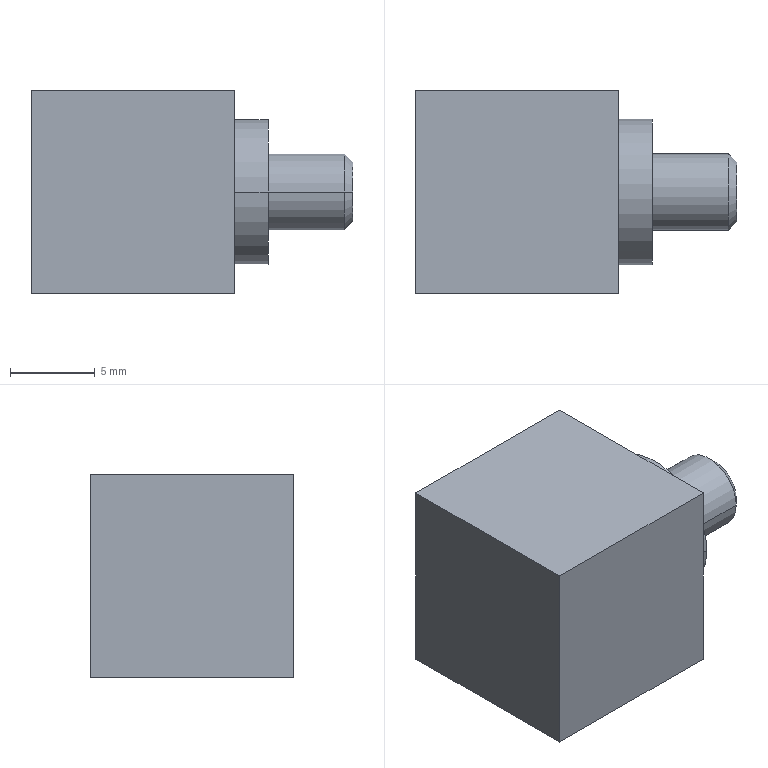Part | STEP file | [LF-A(SUS)]-4 | 1 solid | 23 faces | box 19 x 12 x 12 mm | volume 1287 mm3 | plane 9 | cone 8 | cylinder 6 | commonest cylinder face diameters 4.5 x2 8.6 x2 9.2 x2
STEP:
#1=CARTESIAN_POINT('',(0.,0.,0.));
#2=DIRECTION('',(0.,0.,1.));
#3=DIRECTION('',(1.,0.,0.));
#4=AXIS2_PLACEMENT_3D('',#1,#2,#3);
#5=CARTESIAN_POINT('',(19.,4.25,6.));
#6=VERTEX_POINT('',#5);
#7=CARTESIAN_POINT('',(19.,7.75,6.));
#8=VERTEX_POINT('',#7);
#9=CARTESIAN_POINT('',(19.,6.,6.));
#10=DIRECTION('',(1.,0.,0.));
#11=DIRECTION('',(0.,-1.,0.));
#12=AXIS2_PLACEMENT_3D('',#9,#10,#11);
#13=CIRCLE('',#12,1.75);
#14=CARTESIAN_POINT('',(18.5,6.,6.));
#15=DIRECTION('',(-1.,0.,0.));
#16=DIRECTION('',(0.,1.,0.));
#17=AXIS2_PLACEMENT_3D('',#14,#15,#16);
#18=CONICAL_SURFACE('',#17,2.25,0.7854);
#19=CARTESIAN_POINT('',(3.142,-0.5));
#20=DIRECTION('',(-1.,0.));
#21=VECTOR('',#20,1.);
#22=LINE('',#19,#21);
#23=(GEOMETRIC_REPRESENTATION_CONTEXT(2)PARAMETRIC_REPRESENTATION_CONTEXT()REPRESENTATION_CONTEXT('',''));
#24=DEFINITIONAL_REPRESENTATION('',(#22),#23);
#25=PCURVE('',#18,#24);
#26=CARTESIAN_POINT('',(19.,6.,6.));
#27=DIRECTION('',(1.,0.,0.));
#28=DIRECTION('',(0.,-1.,0.));
#29=AXIS2_PLACEMENT_3D('',#26,#27,#28);
#30=PLANE('',#29);
#31=CARTESIAN_POINT('',(0.,0.));
#32=DIRECTION('',(1.,0.));
#33=AXIS2_PLACEMENT_2D('',#31,#32);
#34=CIRCLE('',#33,1.75);
#35=(GEOMETRIC_REPRESENTATION_CONTEXT(2)PARAMETRIC_REPRESENTATION_CONTEXT()REPRESENTATION_CONTEXT('',''));
#36=DEFINITIONAL_REPRESENTATION('',(#34),#35);
#37=PCURVE('',#30,#36);
#38=SURFACE_CURVE('',#13,(#25,#37),.PCURVE_S1.);
#39=EDGE_CURVE('',#6,#8,#38,.T.);
#40=ORIENTED_EDGE('',*,*,#39,.F.);
#41=CARTESIAN_POINT('',(18.5,3.75,6.));
#42=VERTEX_POINT('',#41);
#43=CARTESIAN_POINT('',(18.5,3.75,6.));
#44=DIRECTION('',(-0.7071,-0.7071,0.));
#45=VECTOR('',#44,1.);
#46=LINE('',#43,#45);
#47=CARTESIAN_POINT('',(3.142,0.));
#48=DIRECTION('',(0.,1.));
#49=VECTOR('',#48,1.);
#50=LINE('',#47,#49);
#51=(GEOMETRIC_REPRESENTATION_CONTEXT(2)PARAMETRIC_REPRESENTATION_CONTEXT()REPRESENTATION_CONTEXT('',''));
#52=DEFINITIONAL_REPRESENTATION('',(#50),#51);
#53=PCURVE('',#18,#52);
#54=CARTESIAN_POINT('',(18.5,6.,6.));
#55=DIRECTION('',(-1.,0.,0.));
#56=DIRECTION('',(0.,1.,0.));
#57=AXIS2_PLACEMENT_3D('',#54,#55,#56);
#58=CONICAL_SURFACE('',#57,2.25,0.7854);
#59=CARTESIAN_POINT('',(3.142,0.));
#60=DIRECTION('',(0.,1.));
#61=VECTOR('',#60,1.);
#62=LINE('',#59,#61);
#63=(GEOMETRIC_REPRESENTATION_CONTEXT(2)PARAMETRIC_REPRESENTATION_CONTEXT()REPRESENTATION_CONTEXT('',''));
#64=DEFINITIONAL_REPRESENTATION('',(#62),#63);
#65=PCURVE('',#58,#64);
#66=SURFACE_CURVE('',#46,(#53,#65),.PCURVE_S1.);
#67=EDGE_CURVE('',#6,#42,#66,.T.);
#68=ORIENTED_EDGE('',*,*,#67,.T.);
#69=CARTESIAN_POINT('',(18.5,8.25,6.));
#70=VERTEX_POINT('',#69);
#71=CARTESIAN_POINT('',(18.5,6.,6.));
#72=DIRECTION('',(-1.,0.,0.));
#73=DIRECTION('',(0.,-1.,0.));
#74=AXIS2_PLACEMENT_3D('',#71,#72,#73);
#75=CIRCLE('',#74,2.25);
#76=CARTESIAN_POINT('',(-3.142,0.));
#77=DIRECTION('',(1.,0.));
#78=VECTOR('',#77,1.);
#79=LINE('',#76,#78);
#80=(GEOMETRIC_REPRESENTATION_CONTEXT(2)PARAMETRIC_REPRESENTATION_CONTEXT()REPRESENTATION_CONTEXT('',''));
#81=DEFINITIONAL_REPRESENTATION('',(#79),#80);
#82=PCURVE('',#18,#81);
#83=CARTESIAN_POINT('',(19.,6.,6.));
#84=DIRECTION('',(-1.,0.,0.));
#85=DIRECTION('',(0.,1.,0.));
#86=AXIS2_PLACEMENT_3D('',#83,#84,#85);
#87=CYLINDRICAL_SURFACE('',#86,2.25);
#88=CARTESIAN_POINT('',(-3.142,0.5));
#89=DIRECTION('',(1.,0.));
#90=VECTOR('',#89,1.);
#91=LINE('',#88,#90);
#92=(GEOMETRIC_REPRESENTATION_CONTEXT(2)PARAMETRIC_REPRESENTATION_CONTEXT()REPRESENTATION_CONTEXT('',''));
#93=DEFINITIONAL_REPRESENTATION('',(#91),#92);
#94=PCURVE('',#87,#93);
#95=SURFACE_CURVE('',#75,(#82,#94),.PCURVE_S1.);
#96=EDGE_CURVE('',#70,#42,#95,.T.);
#97=ORIENTED_EDGE('',*,*,#96,.F.);
#98=CARTESIAN_POINT('',(18.5,8.25,6.));
#99=DIRECTION('',(-0.7071,0.7071,0.));
#100=VECTOR('',#99,1.);
#101=LINE('',#98,#100);
#102=CARTESIAN_POINT('',(0.,0.));
#103=DIRECTION('',(0.,1.));
#104=VECTOR('',#103,1.);
#105=LINE('',#102,#104);
#106=(GEOMETRIC_REPRESENTATION_CONTEXT(2)PARAMETRIC_REPRESENTATION_CONTEXT()REPRESENTATION_CONTEXT('',''));
#107=DEFINITIONAL_REPRESENTATION('',(#105),#106);
#108=PCURVE('',#18,#107);
#109=CARTESIAN_POINT('',(6.283,0.));
#110=DIRECTION('',(0.,1.));
#111=VECTOR('',#110,1.);
#112=LINE('',#109,#111);
#113=(GEOMETRIC_REPRESENTATION_CONTEXT(2)PARAMETRIC_REPRESENTATION_CONTEXT()REPRESENTATION_CONTEXT('',''));
#114=DEFINITIONAL_REPRESENTATION('',(#112),#113);
#115=PCURVE('',#58,#114);
#116=SURFACE_CURVE('',#101,(#108,#115),.PCURVE_S1.);
#117=EDGE_CURVE('',#8,#70,#116,.T.);
#118=ORIENTED_EDGE('',*,*,#117,.F.);
#119=EDGE_LOOP('',(#40,#68,#97,#118));
#120=FACE_BOUND('',#119,.T.);
#121=ADVANCED_FACE('',(#120),#18,.T.);
#122=ORIENTED_EDGE('',*,*,#96,.T.);
#123=CARTESIAN_POINT('',(14.,3.75,6.));
#124=VERTEX_POINT('',#123);
#125=CARTESIAN_POINT('',(19.,3.75,6.));
#126=DIRECTION('',(-1.,0.,0.));
#127=VECTOR('',#126,1.);
#128=LINE('',#125,#127);
#129=CARTESIAN_POINT('',(3.142,0.));
#130=DIRECTION('',(0.,1.));
#131=VECTOR('',#130,1.);
#132=LINE('',#129,#131);
#133=(GEOMETRIC_REPRESENTATION_CONTEXT(2)PARAMETRIC_REPRESENTATION_CONTEXT()REPRESENTATION_CONTEXT('',''));
#134=DEFINITIONAL_REPRESENTATION('',(#132),#133);
#135=PCURVE('',#87,#134);
#136=CARTESIAN_POINT('',(19.,6.,6.));
#137=DIRECTION('',(-1.,0.,0.));
#138=DIRECTION('',(0.,1.,0.));
#139=AXIS2_PLACEMENT_3D('',#136,#137,#138);
#140=CYLINDRICAL_SURFACE('',#139,2.25);
#141=CARTESIAN_POINT('',(3.142,0.));
#142=DIRECTION('',(0.,1.));
#143=VECTOR('',#142,1.);
#144=LINE('',#141,#143);
#145=(GEOMETRIC_REPRESENTATION_CONTEXT(2)PARAMETRIC_REPRESENTATION_CONTEXT()REPRESENTATION_CONTEXT('',''));
#146=DEFINITIONAL_REPRESENTATION('',(#144),#145);
#147=PCURVE('',#140,#146);
#148=SURFACE_CURVE('',#128,(#135,#147),.PCURVE_S1.);
#149=EDGE_CURVE('',#42,#124,#148,.T.);
#150=ORIENTED_EDGE('',*,*,#149,.T.);
#151=CARTESIAN_POINT('',(14.,8.25,6.));
#152=VERTEX_POINT('',#151);
#153=CARTESIAN_POINT('',(14.,6.,6.));
#154=DIRECTION('',(1.,0.,0.));
#155=DIRECTION('',(0.,-1.,0.));
#156=AXIS2_PLACEMENT_3D('',#153,#154,#155);
#157=CIRCLE('',#156,2.25);
#158=CARTESIAN_POINT('',(3.142,5.));
#159=DIRECTION('',(-1.,0.));
#160=VECTOR('',#159,1.);
#161=LINE('',#158,#160);
#162=(GEOMETRIC_REPRESENTATION_CONTEXT(2)PARAMETRIC_REPRESENTATION_CONTEXT()REPRESENTATION_CONTEXT('',''));
#163=DEFINITIONAL_REPRESENTATION('',(#161),#162);
#164=PCURVE('',#87,#163);
#165=CARTESIAN_POINT('',(14.,6.,6.));
#166=DIRECTION('',(1.,0.,0.));
#167=DIRECTION('',(0.,-1.,0.));
#168=AXIS2_PLACEMENT_3D('',#165,#166,#167);
#169=PLANE('',#168);
#170=CARTESIAN_POINT('',(0.,0.));
#171=DIRECTION('',(1.,0.));
#172=AXIS2_PLACEMENT_2D('',#170,#171);
#173=CIRCLE('',#172,2.25);
#174=(GEOMETRIC_REPRESENTATION_CONTEXT(2)PARAMETRIC_REPRESENTATION_CONTEXT()REPRESENTATION_CONTEXT('',''));
#175=DEFINITIONAL_REPRESENTATION('',(#173),#174);
#176=PCURVE('',#169,#175);
#177=SURFACE_CURVE('',#157,(#164,#176),.PCURVE_S1.);
#178=EDGE_CURVE('',#124,#152,#177,.T.);
#179=ORIENTED_EDGE('',*,*,#178,.T.);
#180=CARTESIAN_POINT('',(19.,8.25,6.));
#181=DIRECTION('',(-1.,0.,0.));
#182=VECTOR('',#181,1.);
#183=LINE('',#180,#182);
#184=CARTESIAN_POINT('',(0.,0.));
#185=DIRECTION('',(0.,1.));
#186=VECTOR('',#185,1.);
#187=LINE('',#184,#186);
#188=(GEOMETRIC_REPRESENTATION_CONTEXT(2)PARAMETRIC_REPRESENTATION_CONTEXT()REPRESENTATION_CONTEXT('',''));
#189=DEFINITIONAL_REPRESENTATION('',(#187),#188);
#190=PCURVE('',#87,#189);
#191=CARTESIAN_POINT('',(6.283,0.));
#192=DIRECTION('',(0.,1.));
#193=VECTOR('',#192,1.);
#194=LINE('',#191,#193);
#195=(GEOMETRIC_REPRESENTATION_CONTEXT(2)PARAMETRIC_REPRESENTATION_CONTEXT()REPRESENTATION_CONTEXT('',''));
#196=DEFINITIONAL_REPRESENTATION('',(#194),#195);
#197=PCURVE('',#140,#196);
#198=SURFACE_CURVE('',#183,(#190,#197),.PCURVE_S1.);
#199=EDGE_CURVE('',#70,#152,#198,.T.);
#200=ORIENTED_EDGE('',*,*,#199,.F.);
#201=EDGE_LOOP('',(#122,#150,#179,#200));
#202=FACE_BOUND('',#201,.T.);
#203=ADVANCED_FACE('',(#202),#87,.T.);
#204=CARTESIAN_POINT('',(14.,10.3,6.));
#205=VERTEX_POINT('',#204);
#206=CARTESIAN_POINT('',(14.,1.7,6.));
#207=VERTEX_POINT('',#206);
#208=CARTESIAN_POINT('',(14.,6.,6.));
#209=DIRECTION('',(-1.,0.,0.));
#210=DIRECTION('',(0.,1.,0.));
#211=AXIS2_PLACEMENT_3D('',#208,#209,#210);
#212=CIRCLE('',#211,4.3);
#213=CARTESIAN_POINT('',(14.,6.,6.));
#214=DIRECTION('',(-1.,0.,0.));
#215=DIRECTION('',(0.,1.,0.));
#216=AXIS2_PLACEMENT_3D('',#213,#214,#215);
#217=CYLINDRICAL_SURFACE('',#216,4.3);
#218=CARTESIAN_POINT('',(0.,0.));
#219=DIRECTION('',(1.,0.));
#220=VECTOR('',#219,1.);
#221=LINE('',#218,#220);
#222=(GEOMETRIC_REPRESENTATION_CONTEXT(2)PARAMETRIC_REPRESENTATION_CONTEXT()REPRESENTATION_CONTEXT('',''));
#223=DEFINITIONAL_REPRESENTATION('',(#221),#222);
#224=PCURVE('',#217,#223);
#225=CARTESIAN_POINT('',(-4.3,0.));
#226=CARTESIAN_POINT('',(-4.3,7.448));
#227=CARTESIAN_POINT('',(2.15,3.724));
#228=CARTESIAN_POINT('',(8.6,0.));
#229=CARTESIAN_POINT('',(2.15,-3.724));
#230=CARTESIAN_POINT('',(-4.3,-7.448));
#231=CARTESIAN_POINT('',(-4.3,0.));
#232=(BOUNDED_CURVE()B_SPLINE_CURVE(2,(#225,#226,#227,#228,#229,#230,#231),.UNSPECIFIED.,.T.,.F.)B_SPLINE_CURVE_WITH_KNOTS((1,2,2,2,2,1),(-2.094,0.,2.094,4.189,6.283,8.378),.UNSPECIFIED.)CURVE()GEOMETRIC_REPRESENTATION_ITEM()RATIONAL_B_SPLINE_CURVE((1.,0.5,1.,0.5,1.,0.5,1.))REPRESENTATION_ITEM(''));
#233=(GEOMETRIC_REPRESENTATION_CONTEXT(2)PARAMETRIC_REPRESENTATION_CONTEXT()REPRESENTATION_CONTEXT('',''));
#234=DEFINITIONAL_REPRESENTATION('',(#232),#233);
#235=PCURVE('',#169,#234);
#236=SURFACE_CURVE('',#212,(#224,#235),.PCURVE_S1.);
#237=EDGE_CURVE('',#205,#207,#236,.T.);
#238=ORIENTED_EDGE('',*,*,#237,.T.);
#239=CARTESIAN_POINT('',(12.,1.7,6.));
#240=VERTEX_POINT('',#239);
#241=CARTESIAN_POINT('',(14.,1.7,6.));
#242=DIRECTION('',(-1.,0.,0.));
#243=VECTOR('',#242,1.);
#244=LINE('',#241,#243);
#245=CARTESIAN_POINT('',(3.142,0.));
#246=DIRECTION('',(0.,1.));
#247=VECTOR('',#246,1.);
#248=LINE('',#245,#247);
#249=(GEOMETRIC_REPRESENTATION_CONTEXT(2)PARAMETRIC_REPRESENTATION_CONTEXT()REPRESENTATION_CONTEXT('',''));
#250=DEFINITIONAL_REPRESENTATION('',(#248),#249);
#251=PCURVE('',#217,#250);
#252=CARTESIAN_POINT('',(14.,6.,6.));
#253=DIRECTION('',(-1.,0.,0.));
#254=DIRECTION('',(0.,1.,0.));
#255=AXIS2_PLACEMENT_3D('',#252,#253,#254);
#256=CYLINDRICAL_SURFACE('',#255,4.3);
#257=CARTESIAN_POINT('',(3.142,0.));
#258=DIRECTION('',(0.,1.));
#259=VECTOR('',#258,1.);
#260=LINE('',#257,#259);
#261=(GEOMETRIC_REPRESENTATION_CONTEXT(2)PARAMETRIC_REPRESENTATION_CONTEXT()REPRESENTATION_CONTEXT('',''));
#262=DEFINITIONAL_REPRESENTATION('',(#260),#261);
#263=PCURVE('',#256,#262);
#264=SURFACE_CURVE('',#244,(#251,#263),.PCURVE_S1.);
#265=EDGE_CURVE('',#207,#240,#264,.T.);
#266=ORIENTED_EDGE('',*,*,#265,.T.);
#267=CARTESIAN_POINT('',(12.,10.3,6.));
#268=VERTEX_POINT('',#267);
#269=CARTESIAN_POINT('',(12.,6.,6.));
#270=DIRECTION('',(1.,0.,0.));
#271=DIRECTION('',(0.,-1.,0.));
#272=AXIS2_PLACEMENT_3D('',#269,#270,#271);
#273=CIRCLE('',#272,4.3);
#274=CARTESIAN_POINT('',(3.142,2.));
#275=DIRECTION('',(-1.,0.));
#276=VECTOR('',#275,1.);
#277=LINE('',#274,#276);
#278=(GEOMETRIC_REPRESENTATION_CONTEXT(2)PARAMETRIC_REPRESENTATION_CONTEXT()REPRESENTATION_CONTEXT('',''));
#279=DEFINITIONAL_REPRESENTATION('',(#277),#278);
#280=PCURVE('',#217,#279);
#281=CARTESIAN_POINT('',(12.,6.,6.));
#282=DIRECTION('',(1.,0.,0.));
#283=DIRECTION('',(0.,0.,1.));
#284=AXIS2_PLACEMENT_3D('',#281,#282,#283);
#285=PLANE('',#284);
#286=CARTESIAN_POINT('',(0.,0.));
#287=DIRECTION('',(0.,1.));
#288=AXIS2_PLACEMENT_2D('',#286,#287);
#289=CIRCLE('',#288,4.3);
#290=(GEOMETRIC_REPRESENTATION_CONTEXT(2)PARAMETRIC_REPRESENTATION_CONTEXT()REPRESENTATION_CONTEXT('',''));
#291=DEFINITIONAL_REPRESENTATION('',(#289),#290);
#292=PCURVE('',#285,#291);
#293=SURFACE_CURVE('',#273,(#280,#292),.PCURVE_S1.);
#294=EDGE_CURVE('',#240,#268,#293,.T.);
#295=ORIENTED_EDGE('',*,*,#294,.T.);
#296=CARTESIAN_POINT('',(14.,10.3,6.));
#297=DIRECTION('',(-1.,0.,0.));
#298=VECTOR('',#297,1.);
#299=LINE('',#296,#298);
#300=CARTESIAN_POINT('',(0.,0.));
#301=DIRECTION('',(0.,1.));
#302=VECTOR('',#301,1.);
#303=LINE('',#300,#302);
#304=(GEOMETRIC_REPRESENTATION_CONTEXT(2)PARAMETRIC_REPRESENTATION_CONTEXT()REPRESENTATION_CONTEXT('',''));
#305=DEFINITIONAL_REPRESENTATION('',(#303),#304);
#306=PCURVE('',#217,#305);
#307=CARTESIAN_POINT('',(6.283,0.));
#308=DIRECTION('',(0.,1.));
#309=VECTOR('',#308,1.);
#310=LINE('',#307,#309);
#311=(GEOMETRIC_REPRESENTATION_CONTEXT(2)PARAMETRIC_REPRESENTATION_CONTEXT()REPRESENTATION_CONTEXT('',''));
#312=DEFINITIONAL_REPRESENTATION('',(#310),#311);
#313=PCURVE('',#256,#312);
#314=SURFACE_CURVE('',#299,(#306,#313),.PCURVE_S1.);
#315=EDGE_CURVE('',#205,#268,#314,.T.);
#316=ORIENTED_EDGE('',*,*,#315,.F.);
#317=EDGE_LOOP('',(#238,#266,#295,#316));
#318=FACE_BOUND('',#317,.T.);
#319=ADVANCED_FACE('',(#318),#217,.T.);
#320=CARTESIAN_POINT('',(1.419,3.552,6.422));
#321=VERTEX_POINT('',#320);
#322=CARTESIAN_POINT('',(1.294,7.567,6.434));
#323=VERTEX_POINT('',#322);
#324=CARTESIAN_POINT('',(1.157,12.,6.446));
#325=DIRECTION('',(-0.0311,0.9995,0.002866));
#326=VECTOR('',#325,1.);
#327=LINE('',#324,#326);
#328=CARTESIAN_POINT('',(6.,12.,6.));
#329=DIRECTION('',(0.,1.,0.));
#330=DIRECTION('',(-0.9958,0.,0.09176));
#331=AXIS2_PLACEMENT_3D('',#328,#329,#330);
#332=CONICAL_SURFACE('',#331,4.864,0.03124);
#333=CARTESIAN_POINT('',(6.283,0.));
#334=DIRECTION('',(0.,1.));
#335=VECTOR('',#334,1.);
#336=LINE('',#333,#335);
#337=(GEOMETRIC_REPRESENTATION_CONTEXT(2)PARAMETRIC_REPRESENTATION_CONTEXT()REPRESENTATION_CONTEXT('',''));
#338=DEFINITIONAL_REPRESENTATION('',(#336),#337);
#339=PCURVE('',#332,#338);
#340=CARTESIAN_POINT('',(6.,12.,6.));
#341=DIRECTION('',(0.,1.,0.));
#342=DIRECTION('',(-0.9958,0.,0.09176));
#343=AXIS2_PLACEMENT_3D('',#340,#341,#342);
#344=CONICAL_SURFACE('',#343,4.864,0.03124);
#345=CARTESIAN_POINT('',(0.,0.));
#346=DIRECTION('',(0.,1.));
#347=VECTOR('',#346,1.);
#348=LINE('',#345,#347);
#349=(GEOMETRIC_REPRESENTATION_CONTEXT(2)PARAMETRIC_REPRESENTATION_CONTEXT()REPRESENTATION_CONTEXT('',''));
#350=DEFINITIONAL_REPRESENTATION('',(#348),#349);
#351=PCURVE('',#344,#350);
#352=SURFACE_CURVE('',#327,(#339,#351),.PCURVE_S1.);
#353=EDGE_CURVE('',#321,#323,#352,.T.);
#354=ORIENTED_EDGE('',*,*,#353,.T.);
#355=CARTESIAN_POINT('',(1.275,7.567,6.));
#356=VERTEX_POINT('',#355);
#357=CARTESIAN_POINT('',(6.,7.567,6.));
#358=DIRECTION('',(0.,-1.,0.));
#359=DIRECTION('',(1.,0.,0.));
#360=AXIS2_PLACEMENT_3D('',#357,#358,#359);
#361=CIRCLE('',#360,4.725);
#362=CARTESIAN_POINT('',(9.333,-4.433));
#363=DIRECTION('',(-1.,0.));
#364=VECTOR('',#363,1.);
#365=LINE('',#362,#364);
#366=(GEOMETRIC_REPRESENTATION_CONTEXT(2)PARAMETRIC_REPRESENTATION_CONTEXT()REPRESENTATION_CONTEXT('',''));
#367=DEFINITIONAL_REPRESENTATION('',(#365),#366);
#368=PCURVE('',#332,#367);
#369=CARTESIAN_POINT('',(6.,7.,6.));
#370=DIRECTION('',(0.,1.,0.));
#371=DIRECTION('',(-1.,0.,0.));
#372=AXIS2_PLACEMENT_3D('',#369,#370,#371);
#373=CONICAL_SURFACE('',#372,4.158,0.7854);
#374=CARTESIAN_POINT('',(3.142,0.5674));
#375=DIRECTION('',(-1.,0.));
#376=VECTOR('',#375,1.);
#377=LINE('',#374,#376);
#378=(GEOMETRIC_REPRESENTATION_CONTEXT(2)PARAMETRIC_REPRESENTATION_CONTEXT()REPRESENTATION_CONTEXT('',''));
#379=DEFINITIONAL_REPRESENTATION('',(#377),#378);
#380=PCURVE('',#373,#379);
#381=SURFACE_CURVE('',#361,(#368,#380),.PCURVE_S1.);
#382=EDGE_CURVE('',#323,#356,#381,.T.);
#383=ORIENTED_EDGE('',*,*,#382,.T.);
#384=CARTESIAN_POINT('',(10.706,7.567,5.566));
#385=VERTEX_POINT('',#384);
#386=CARTESIAN_POINT('',(6.,7.567,6.));
#387=DIRECTION('',(0.,-1.,0.));
#388=DIRECTION('',(1.,0.,0.));
#389=AXIS2_PLACEMENT_3D('',#386,#387,#388);
#390=CIRCLE('',#389,4.725);
#391=CARTESIAN_POINT('',(9.333,-4.433));
#392=DIRECTION('',(-1.,0.));
#393=VECTOR('',#392,1.);
#394=LINE('',#391,#393);
#395=(GEOMETRIC_REPRESENTATION_CONTEXT(2)PARAMETRIC_REPRESENTATION_CONTEXT()REPRESENTATION_CONTEXT('',''));
#396=DEFINITIONAL_REPRESENTATION('',(#394),#395);
#397=PCURVE('',#332,#396);
#398=CARTESIAN_POINT('',(6.,7.,6.));
#399=DIRECTION('',(0.,1.,0.));
#400=DIRECTION('',(-1.,0.,0.));
#401=AXIS2_PLACEMENT_3D('',#398,#399,#400);
#402=CONICAL_SURFACE('',#401,4.158,0.7854);
#403=CARTESIAN_POINT('',(9.425,0.5674));
#404=DIRECTION('',(-1.,0.));
#405=VECTOR('',#404,1.);
#406=LINE('',#403,#405);
#407=(GEOMETRIC_REPRESENTATION_CONTEXT(2)PARAMETRIC_REPRESENTATION_CONTEXT()REPRESENTATION_CONTEXT('',''));
#408=DEFINITIONAL_REPRESENTATION('',(#406),#407);
#409=PCURVE('',#402,#408);
#410=SURFACE_CURVE('',#390,(#397,#409),.PCURVE_S1.);
#411=EDGE_CURVE('',#356,#385,#410,.T.);
#412=ORIENTED_EDGE('',*,*,#411,.T.);
#413=CARTESIAN_POINT('',(10.581,3.552,5.578));
#414=VERTEX_POINT('',#413);
#415=CARTESIAN_POINT('',(10.843,12.,5.554));
#416=DIRECTION('',(0.0311,0.9995,-0.002866));
#417=VECTOR('',#416,1.);
#418=LINE('',#415,#417);
#419=CARTESIAN_POINT('',(3.142,0.));
#420=DIRECTION('',(0.,1.));
#421=VECTOR('',#420,1.);
#422=LINE('',#419,#421);
#423=(GEOMETRIC_REPRESENTATION_CONTEXT(2)PARAMETRIC_REPRESENTATION_CONTEXT()REPRESENTATION_CONTEXT('',''));
#424=DEFINITIONAL_REPRESENTATION('',(#422),#423);
#425=PCURVE('',#332,#424);
#426=CARTESIAN_POINT('',(3.142,0.));
#427=DIRECTION('',(0.,1.));
#428=VECTOR('',#427,1.);
#429=LINE('',#426,#428);
#430=(GEOMETRIC_REPRESENTATION_CONTEXT(2)PARAMETRIC_REPRESENTATION_CONTEXT()REPRESENTATION_CONTEXT('',''));
#431=DEFINITIONAL_REPRESENTATION('',(#429),#430);
#432=PCURVE('',#344,#431);
#433=SURFACE_CURVE('',#418,(#425,#432),.PCURVE_S1.);
#434=EDGE_CURVE('',#414,#385,#433,.T.);
#435=ORIENTED_EDGE('',*,*,#434,.F.);
#436=CARTESIAN_POINT('',(6.,3.552,6.));
#437=DIRECTION('',(0.,1.,0.));
#438=DIRECTION('',(-0.9958,0.,0.09176));
#439=AXIS2_PLACEMENT_3D('',#436,#437,#438);
#440=CIRCLE('',#439,4.6);
#441=CARTESIAN_POINT('',(0.,-8.448));
#442=DIRECTION('',(1.,0.));
#443=VECTOR('',#442,1.);
#444=LINE('',#441,#443);
#445=(GEOMETRIC_REPRESENTATION_CONTEXT(2)PARAMETRIC_REPRESENTATION_CONTEXT()REPRESENTATION_CONTEXT('',''));
#446=DEFINITIONAL_REPRESENTATION('',(#444),#445);
#447=PCURVE('',#332,#446);
#448=CARTESIAN_POINT('',(6.,12.,6.));
#449=DIRECTION('',(0.,1.,0.));
#450=DIRECTION('',(-0.9958,0.,0.09176));
#451=AXIS2_PLACEMENT_3D('',#448,#449,#450);
#452=CYLINDRICAL_SURFACE('',#451,4.6);
#453=CARTESIAN_POINT('',(0.,-8.448));
#454=DIRECTION('',(1.,0.));
#455=VECTOR('',#454,1.);
#456=LINE('',#453,#455);
#457=(GEOMETRIC_REPRESENTATION_CONTEXT(2)PARAMETRIC_REPRESENTATION_CONTEXT()REPRESENTATION_CONTEXT('',''));
#458=DEFINITIONAL_REPRESENTATION('',(#456),#457);
#459=PCURVE('',#452,#458);
#460=SURFACE_CURVE('',#440,(#447,#459),.PCURVE_S1.);
#461=EDGE_CURVE('',#414,#321,#460,.T.);
#462=ORIENTED_EDGE('',*,*,#461,.T.);
#463=EDGE_LOOP('',(#354,#383,#412,#435,#462));
#464=FACE_BOUND('',#463,.F.);
#465=ADVANCED_FACE('',(#464),#332,.F.);
#466=CARTESIAN_POINT('',(1.419,3.,6.422));
#467=VERTEX_POINT('',#466);
#468=CARTESIAN_POINT('',(1.419,12.,6.422));
#469=DIRECTION('',(0.,1.,0.));
#470=VECTOR('',#469,1.);
#471=LINE('',#468,#470);
#472=CARTESIAN_POINT('',(6.283,0.));
#473=DIRECTION('',(0.,1.));
#474=VECTOR('',#473,1.);
#475=LINE('',#472,#474);
#476=(GEOMETRIC_REPRESENTATION_CONTEXT(2)PARAMETRIC_REPRESENTATION_CONTEXT()REPRESENTATION_CONTEXT('',''));
#477=DEFINITIONAL_REPRESENTATION('',(#475),#476);
#478=PCURVE('',#452,#477);
#479=CARTESIAN_POINT('',(6.,12.,6.));
#480=DIRECTION('',(0.,1.,0.));
#481=DIRECTION('',(-0.9958,0.,0.09176));
#482=AXIS2_PLACEMENT_3D('',#479,#480,#481);
#483=CYLINDRICAL_SURFACE('',#482,4.6);
#484=CARTESIAN_POINT('',(0.,0.));
#485=DIRECTION('',(0.,1.));
#486=VECTOR('',#485,1.);
#487=LINE('',#484,#486);
#488=(GEOMETRIC_REPRESENTATION_CONTEXT(2)PARAMETRIC_REPRESENTATION_CONTEXT()REPRESENTATION_CONTEXT('',''));
#489=DEFINITIONAL_REPRESENTATION('',(#487),#488);
#490=PCURVE('',#483,#489);
#491=SURFACE_CURVE('',#471,(#478,#490),.PCURVE_S1.);
#492=EDGE_CURVE('',#467,#321,#491,.T.);
#493=ORIENTED_EDGE('',*,*,#492,.T.);
#494=ORIENTED_EDGE('',*,*,#461,.F.);
#495=CARTESIAN_POINT('',(10.581,3.,5.578));
#496=VERTEX_POINT('',#495);
#497=CARTESIAN_POINT('',(10.581,12.,5.578));
#498=DIRECTION('',(0.,1.,0.));
#499=VECTOR('',#498,1.);
#500=LINE('',#497,#499);
#501=CARTESIAN_POINT('',(3.142,0.));
#502=DIRECTION('',(0.,1.));
#503=VECTOR('',#502,1.);
#504=LINE('',#501,#503);
#505=(GEOMETRIC_REPRESENTATION_CONTEXT(2)PARAMETRIC_REPRESENTATION_CONTEXT()REPRESENTATION_CONTEXT('',''));
#506=DEFINITIONAL_REPRESENTATION('',(#504),#505);
#507=PCURVE('',#452,#506);
#508=CARTESIAN_POINT('',(3.142,0.));
#509=DIRECTION('',(0.,1.));
#510=VECTOR('',#509,1.);
#511=LINE('',#508,#510);
#512=(GEOMETRIC_REPRESENTATION_CONTEXT(2)PARAMETRIC_REPRESENTATION_CONTEXT()REPRESENTATION_CONTEXT('',''));
#513=DEFINITIONAL_REPRESENTATION('',(#511),#512);
#514=PCURVE('',#483,#513);
#515=SURFACE_CURVE('',#500,(#507,#514),.PCURVE_S1.);
#516=EDGE_CURVE('',#496,#414,#515,.T.);
#517=ORIENTED_EDGE('',*,*,#516,.F.);
#518=CARTESIAN_POINT('',(6.,3.,6.));
#519=DIRECTION('',(0.,-1.,0.));
#520=DIRECTION('',(1.,0.,0.));
#521=AXIS2_PLACEMENT_3D('',#518,#519,#520);
#522=CIRCLE('',#521,4.6);
#523=CARTESIAN_POINT('',(9.333,-9.));
#524=DIRECTION('',(-1.,0.));
#525=VECTOR('',#524,1.);
#526=LINE('',#523,#525);
#527=(GEOMETRIC_REPRESENTATION_CONTEXT(2)PARAMETRIC_REPRESENTATION_CONTEXT()REPRESENTATION_CONTEXT('',''));
#528=DEFINITIONAL_REPRESENTATION('',(#526),#527);
#529=PCURVE('',#452,#528);
#530=CARTESIAN_POINT('',(6.,3.,6.));
#531=DIRECTION('',(0.,1.,0.));
#532=DIRECTION('',(1.,0.,0.));
#533=AXIS2_PLACEMENT_3D('',#530,#531,#532);
#534=PLANE('',#533);
#535=CARTESIAN_POINT('',(4.6,0.));
#536=CARTESIAN_POINT('',(4.6,-7.967));
#537=CARTESIAN_POINT('',(-2.3,-3.984));
#538=CARTESIAN_POINT('',(-9.2,0.));
#539=CARTESIAN_POINT('',(-2.3,3.984));
#540=CARTESIAN_POINT('',(4.6,7.967));
#541=CARTESIAN_POINT('',(4.6,0.));
#542=(BOUNDED_CURVE()B_SPLINE_CURVE(2,(#535,#536,#537,#538,#539,#540,#541),.UNSPECIFIED.,.T.,.F.)B_SPLINE_CURVE_WITH_KNOTS((1,2,2,2,2,1),(-2.094,0.,2.094,4.189,6.283,8.378),.UNSPECIFIED.)CURVE()GEOMETRIC_REPRESENTATION_ITEM()RATIONAL_B_SPLINE_CURVE((1.,0.5,1.,0.5,1.,0.5,1.))REPRESENTATION_ITEM(''));
#543=(GEOMETRIC_REPRESENTATION_CONTEXT(2)PARAMETRIC_REPRESENTATION_CONTEXT()REPRESENTATION_CONTEXT('',''));
#544=DEFINITIONAL_REPRESENTATION('',(#542),#543);
#545=PCURVE('',#534,#544);
#546=SURFACE_CURVE('',#522,(#529,#545),.PCURVE_S1.);
#547=EDGE_CURVE('',#467,#496,#546,.T.);
#548=ORIENTED_EDGE('',*,*,#547,.F.);
#549=EDGE_LOOP('',(#493,#494,#517,#548));
#550=FACE_BOUND('',#549,.F.);
#551=ADVANCED_FACE('',(#550),#452,.F.);
#552=CARTESIAN_POINT('',(1.242,7.6,6.));
#553=VERTEX_POINT('',#552);
#554=CARTESIAN_POINT('',(1.105,12.,6.));
#555=VERTEX_POINT('',#554);
#556=CARTESIAN_POINT('',(1.242,7.6,6.));
#557=DIRECTION('',(-0.0312,0.9995,0.));
#558=VECTOR('',#557,1.);
#559=LINE('',#556,#558);
#560=CARTESIAN_POINT('',(6.,7.6,6.));
#561=DIRECTION('',(0.,1.,0.));
#562=DIRECTION('',(-1.,0.,0.));
#563=AXIS2_PLACEMENT_3D('',#560,#561,#562);
#564=CONICAL_SURFACE('',#563,4.758,0.03121);
#565=CARTESIAN_POINT('',(6.283,0.));
#566=DIRECTION('',(0.,1.));
#567=VECTOR('',#566,1.);
#568=LINE('',#565,#567);
#569=(GEOMETRIC_REPRESENTATION_CONTEXT(2)PARAMETRIC_REPRESENTATION_CONTEXT()REPRESENTATION_CONTEXT('',''));
#570=DEFINITIONAL_REPRESENTATION('',(#568),#569);
#571=PCURVE('',#564,#570);
#572=CARTESIAN_POINT('',(6.,7.6,6.));
#573=DIRECTION('',(0.,1.,0.));
#574=DIRECTION('',(-1.,0.,0.));
#575=AXIS2_PLACEMENT_3D('',#572,#573,#574);
#576=CONICAL_SURFACE('',#575,4.758,0.03121);
#577=CARTESIAN_POINT('',(0.,0.));
#578=DIRECTION('',(0.,1.));
#579=VECTOR('',#578,1.);
#580=LINE('',#577,#579);
#581=(GEOMETRIC_REPRESENTATION_CONTEXT(2)PARAMETRIC_REPRESENTATION_CONTEXT()REPRESENTATION_CONTEXT('',''));
#582=DEFINITIONAL_REPRESENTATION('',(#580),#581);
#583=PCURVE('',#576,#582);
#584=SURFACE_CURVE('',#559,(#571,#583),.PCURVE_S1.);
#585=EDGE_CURVE('',#553,#555,#584,.T.);
#586=ORIENTED_EDGE('',*,*,#585,.T.);
#587=CARTESIAN_POINT('',(10.895,12.,6.));
#588=VERTEX_POINT('',#587);
#589=CARTESIAN_POINT('',(6.,12.,6.));
#590=DIRECTION('',(0.,-1.,0.));
#591=DIRECTION('',(0.,0.,1.));
#592=AXIS2_PLACEMENT_3D('',#589,#590,#591);
#593=CIRCLE('',#592,4.895);
#594=CARTESIAN_POINT('',(7.854,4.4));
#595=DIRECTION('',(-1.,0.));
#596=VECTOR('',#595,1.);
#597=LINE('',#594,#596);
#598=(GEOMETRIC_REPRESENTATION_CONTEXT(2)PARAMETRIC_REPRESENTATION_CONTEXT()REPRESENTATION_CONTEXT('',''));
#599=DEFINITIONAL_REPRESENTATION('',(#597),#598);
#600=PCURVE('',#564,#599);
#601=CARTESIAN_POINT('',(12.,12.,6.));
#602=DIRECTION('',(0.,1.,0.));
#603=DIRECTION('',(1.,0.,0.));
#604=AXIS2_PLACEMENT_3D('',#601,#602,#603);
#605=PLANE('',#604);
#606=CARTESIAN_POINT('',(-6.,-4.895));
#607=CARTESIAN_POINT('',(-14.479,-4.895));
#608=CARTESIAN_POINT('',(-10.239,2.448));
#609=CARTESIAN_POINT('',(-6.,9.79));
#610=CARTESIAN_POINT('',(-1.761,2.448));
#611=CARTESIAN_POINT('',(2.479,-4.895));
#612=CARTESIAN_POINT('',(-6.,-4.895));
#613=(BOUNDED_CURVE()B_SPLINE_CURVE(2,(#606,#607,#608,#609,#610,#611,#612),.UNSPECIFIED.,.T.,.F.)B_SPLINE_CURVE_WITH_KNOTS((1,2,2,2,2,1),(-2.094,0.,2.094,4.189,6.283,8.378),.UNSPECIFIED.)CURVE()GEOMETRIC_REPRESENTATION_ITEM()RATIONAL_B_SPLINE_CURVE((1.,0.5,1.,0.5,1.,0.5,1.))REPRESENTATION_ITEM(''));
#614=(GEOMETRIC_REPRESENTATION_CONTEXT(2)PARAMETRIC_REPRESENTATION_CONTEXT()REPRESENTATION_CONTEXT('',''));
#615=DEFINITIONAL_REPRESENTATION('',(#613),#614);
#616=PCURVE('',#605,#615);
#617=SURFACE_CURVE('',#593,(#600,#616),.PCURVE_S1.);
#618=EDGE_CURVE('',#555,#588,#617,.T.);
#619=ORIENTED_EDGE('',*,*,#618,.T.);
#620=CARTESIAN_POINT('',(10.758,7.6,6.));
#621=VERTEX_POINT('',#620);
#622=CARTESIAN_POINT('',(10.758,7.6,6.));
#623=DIRECTION('',(0.0312,0.9995,0.));
#624=VECTOR('',#623,1.);
#625=LINE('',#622,#624);
#626=CARTESIAN_POINT('',(3.142,0.));
#627=DIRECTION('',(0.,1.));
#628=VECTOR('',#627,1.);
#629=LINE('',#626,#628);
#630=(GEOMETRIC_REPRESENTATION_CONTEXT(2)PARAMETRIC_REPRESENTATION_CONTEXT()REPRESENTATION_CONTEXT('',''));
#631=DEFINITIONAL_REPRESENTATION('',(#629),#630);
#632=PCURVE('',#564,#631);
#633=CARTESIAN_POINT('',(3.142,0.));
#634=DIRECTION('',(0.,1.));
#635=VECTOR('',#634,1.);
#636=LINE('',#633,#635);
#637=(GEOMETRIC_REPRESENTATION_CONTEXT(2)PARAMETRIC_REPRESENTATION_CONTEXT()REPRESENTATION_CONTEXT('',''));
#638=DEFINITIONAL_REPRESENTATION('',(#636),#637);
#639=PCURVE('',#576,#638);
#640=SURFACE_CURVE('',#625,(#632,#639),.PCURVE_S1.);
#641=EDGE_CURVE('',#621,#588,#640,.T.);
#642=ORIENTED_EDGE('',*,*,#641,.F.);
#643=CARTESIAN_POINT('',(6.,7.6,6.));
#644=DIRECTION('',(0.,-1.,0.));
#645=DIRECTION('',(1.,0.,0.));
#646=AXIS2_PLACEMENT_3D('',#643,#644,#645);
#647=CIRCLE('',#646,4.758);
#648=CARTESIAN_POINT('',(9.425,0.));
#649=DIRECTION('',(-1.,0.));
#650=VECTOR('',#649,1.);
#651=LINE('',#648,#650);
#652=(GEOMETRIC_REPRESENTATION_CONTEXT(2)PARAMETRIC_REPRESENTATION_CONTEXT()REPRESENTATION_CONTEXT('',''));
#653=DEFINITIONAL_REPRESENTATION('',(#651),#652);
#654=PCURVE('',#564,#653);
#655=CARTESIAN_POINT('',(9.425,0.5997));
#656=DIRECTION('',(-1.,0.));
#657=VECTOR('',#656,1.);
#658=LINE('',#655,#657);
#659=(GEOMETRIC_REPRESENTATION_CONTEXT(2)PARAMETRIC_REPRESENTATION_CONTEXT()REPRESENTATION_CONTEXT('',''));
#660=DEFINITIONAL_REPRESENTATION('',(#658),#659);
#661=PCURVE('',#402,#660);
#662=SURFACE_CURVE('',#647,(#654,#661),.PCURVE_S1.);
#663=EDGE_CURVE('',#553,#621,#662,.T.);
#664=ORIENTED_EDGE('',*,*,#663,.F.);
#665=EDGE_LOOP('',(#586,#619,#642,#664));
#666=FACE_BOUND('',#665,.F.);
#667=ADVANCED_FACE('',(#666),#564,.F.);
#668=CARTESIAN_POINT('',(1.842,7.,6.));
#669=DIRECTION('',(-0.7071,0.7071,0.));
#670=VECTOR('',#669,1.);
#671=LINE('',#668,#670);
#672=CARTESIAN_POINT('',(6.283,0.));
#673=DIRECTION('',(0.,1.));
#674=VECTOR('',#673,1.);
#675=LINE('',#672,#674);
#676=(GEOMETRIC_REPRESENTATION_CONTEXT(2)PARAMETRIC_REPRESENTATION_CONTEXT()REPRESENTATION_CONTEXT('',''));
#677=DEFINITIONAL_REPRESENTATION('',(#675),#676);
#678=PCURVE('',#402,#677);
#679=CARTESIAN_POINT('',(0.,0.));
#680=DIRECTION('',(0.,1.));
#681=VECTOR('',#680,1.);
#682=LINE('',#679,#681);
#683=(GEOMETRIC_REPRESENTATION_CONTEXT(2)PARAMETRIC_REPRESENTATION_CONTEXT()REPRESENTATION_CONTEXT('',''));
#684=DEFINITIONAL_REPRESENTATION('',(#682),#683);
#685=PCURVE('',#373,#684);
#686=SURFACE_CURVE('',#671,(#678,#685),.PCURVE_S1.);
#687=EDGE_CURVE('',#356,#553,#686,.T.);
#688=ORIENTED_EDGE('',*,*,#687,.T.);
#689=ORIENTED_EDGE('',*,*,#663,.T.);
#690=CARTESIAN_POINT('',(10.725,7.567,6.));
#691=VERTEX_POINT('',#690);
#692=CARTESIAN_POINT('',(10.158,7.,6.));
#693=DIRECTION('',(0.7071,0.7071,0.));
#694=VECTOR('',#693,1.);
#695=LINE('',#692,#694);
#696=CARTESIAN_POINT('',(3.142,0.));
#697=DIRECTION('',(0.,1.));
#698=VECTOR('',#697,1.);
#699=LINE('',#696,#698);
#700=(GEOMETRIC_REPRESENTATION_CONTEXT(2)PARAMETRIC_REPRESENTATION_CONTEXT()REPRESENTATION_CONTEXT('',''));
#701=DEFINITIONAL_REPRESENTATION('',(#699),#700);
#702=PCURVE('',#402,#701);
#703=CARTESIAN_POINT('',(3.142,0.));
#704=DIRECTION('',(0.,1.));
#705=VECTOR('',#704,1.);
#706=LINE('',#703,#705);
#707=(GEOMETRIC_REPRESENTATION_CONTEXT(2)PARAMETRIC_REPRESENTATION_CONTEXT()REPRESENTATION_CONTEXT('',''));
#708=DEFINITIONAL_REPRESENTATION('',(#706),#707);
#709=PCURVE('',#373,#708);
#710=SURFACE_CURVE('',#695,(#702,#709),.PCURVE_S1.);
#711=EDGE_CURVE('',#691,#621,#710,.T.);
#712=ORIENTED_EDGE('',*,*,#711,.F.);
#713=CARTESIAN_POINT('',(6.,7.567,6.));
#714=DIRECTION('',(0.,-1.,0.));
#715=DIRECTION('',(1.,0.,0.));
#716=AXIS2_PLACEMENT_3D('',#713,#714,#715);
#717=CIRCLE('',#716,4.725);
#718=CARTESIAN_POINT('',(9.425,0.5674));
#719=DIRECTION('',(-1.,0.));
#720=VECTOR('',#719,1.);
#721=LINE('',#718,#720);
#722=(GEOMETRIC_REPRESENTATION_CONTEXT(2)PARAMETRIC_REPRESENTATION_CONTEXT()REPRESENTATION_CONTEXT('',''));
#723=DEFINITIONAL_REPRESENTATION('',(#721),#722);
#724=PCURVE('',#402,#723);
#725=CARTESIAN_POINT('',(9.333,-4.433));
#726=DIRECTION('',(-1.,0.));
#727=VECTOR('',#726,1.);
#728=LINE('',#725,#727);
#729=(GEOMETRIC_REPRESENTATION_CONTEXT(2)PARAMETRIC_REPRESENTATION_CONTEXT()REPRESENTATION_CONTEXT('',''));
#730=DEFINITIONAL_REPRESENTATION('',(#728),#729);
#731=PCURVE('',#344,#730);
#732=SURFACE_CURVE('',#717,(#724,#731),.PCURVE_S1.);
#733=EDGE_CURVE('',#385,#691,#732,.T.);
#734=ORIENTED_EDGE('',*,*,#733,.F.);
#735=ORIENTED_EDGE('',*,*,#411,.F.);
#736=EDGE_LOOP('',(#688,#689,#712,#734,#735));
#737=FACE_BOUND('',#736,.F.);
#738=ADVANCED_FACE('',(#737),#402,.F.);
#739=CARTESIAN_POINT('',(0.,12.,0.));
#740=VERTEX_POINT('',#739);
#741=CARTESIAN_POINT('',(0.,12.,12.));
#742=VERTEX_POINT('',#741);
#743=CARTESIAN_POINT('',(0.,12.,6.));
#744=DIRECTION('',(0.,0.,1.));
#745=VECTOR('',#744,1.);
#746=LINE('',#743,#745);
#747=CARTESIAN_POINT('',(0.,6.,6.));
#748=DIRECTION('',(-1.,0.,0.));
#749=DIRECTION('',(0.,0.,-1.));
#750=AXIS2_PLACEMENT_3D('',#747,#748,#749);
#751=PLANE('',#750);
#752=CARTESIAN_POINT('',(0.,-6.));
#753=DIRECTION('',(-1.,0.));
#754=VECTOR('',#753,1.);
#755=LINE('',#752,#754);
#756=(GEOMETRIC_REPRESENTATION_CONTEXT(2)PARAMETRIC_REPRESENTATION_CONTEXT()REPRESENTATION_CONTEXT('',''));
#757=DEFINITIONAL_REPRESENTATION('',(#755),#756);
#758=PCURVE('',#751,#757);
#759=CARTESIAN_POINT('',(-12.,0.));
#760=DIRECTION('',(0.,-1.));
#761=VECTOR('',#760,1.);
#762=LINE('',#759,#761);
#763=(GEOMETRIC_REPRESENTATION_CONTEXT(2)PARAMETRIC_REPRESENTATION_CONTEXT()REPRESENTATION_CONTEXT('',''));
#764=DEFINITIONAL_REPRESENTATION('',(#762),#763);
#765=PCURVE('',#605,#764);
#766=SURFACE_CURVE('',#746,(#758,#765),.PCURVE_S1.);
#767=EDGE_CURVE('',#740,#742,#766,.T.);
#768=ORIENTED_EDGE('',*,*,#767,.F.);
#769=CARTESIAN_POINT('',(0.,0.,0.));
#770=VERTEX_POINT('',#769);
#771=CARTESIAN_POINT('',(0.,6.,0.));
#772=DIRECTION('',(0.,1.,0.));
#773=VECTOR('',#772,1.);
#774=LINE('',#771,#773);
#775=CARTESIAN_POINT('',(6.,0.));
#776=DIRECTION('',(0.,-1.));
#777=VECTOR('',#776,1.);
#778=LINE('',#775,#777);
#779=(GEOMETRIC_REPRESENTATION_CONTEXT(2)PARAMETRIC_REPRESENTATION_CONTEXT()REPRESENTATION_CONTEXT('',''));
#780=DEFINITIONAL_REPRESENTATION('',(#778),#779);
#781=PCURVE('',#751,#780);
#782=CARTESIAN_POINT('',(12.,6.,0.));
#783=DIRECTION('',(0.,0.,-1.));
#784=DIRECTION('',(1.,0.,0.));
#785=AXIS2_PLACEMENT_3D('',#782,#783,#784);
#786=PLANE('',#785);
#787=CARTESIAN_POINT('',(-12.,0.));
#788=DIRECTION('',(0.,-1.));
#789=VECTOR('',#788,1.);
#790=LINE('',#787,#789);
#791=(GEOMETRIC_REPRESENTATION_CONTEXT(2)PARAMETRIC_REPRESENTATION_CONTEXT()REPRESENTATION_CONTEXT('',''));
#792=DEFINITIONAL_REPRESENTATION('',(#790),#791);
#793=PCURVE('',#786,#792);
#794=SURFACE_CURVE('',#774,(#781,#793),.PCURVE_S1.);
#795=EDGE_CURVE('',#770,#740,#794,.T.);
#796=ORIENTED_EDGE('',*,*,#795,.F.);
#797=CARTESIAN_POINT('',(0.,0.,12.));
#798=VERTEX_POINT('',#797);
#799=CARTESIAN_POINT('',(0.,0.,6.));
#800=DIRECTION('',(0.,0.,-1.));
#801=VECTOR('',#800,1.);
#802=LINE('',#799,#801);
#803=CARTESIAN_POINT('',(0.,6.));
#804=DIRECTION('',(1.,0.));
#805=VECTOR('',#804,1.);
#806=LINE('',#803,#805);
#807=(GEOMETRIC_REPRESENTATION_CONTEXT(2)PARAMETRIC_REPRESENTATION_CONTEXT()REPRESENTATION_CONTEXT('',''));
#808=DEFINITIONAL_REPRESENTATION('',(#806),#807);
#809=PCURVE('',#751,#808);
#810=CARTESIAN_POINT('',(12.,0.,6.));
#811=DIRECTION('',(0.,-1.,0.));
#812=DIRECTION('',(-1.,0.,0.));
#813=AXIS2_PLACEMENT_3D('',#810,#811,#812);
#814=PLANE('',#813);
#815=CARTESIAN_POINT('',(12.,0.));
#816=DIRECTION('',(0.,1.));
#817=VECTOR('',#816,1.);
#818=LINE('',#815,#817);
#819=(GEOMETRIC_REPRESENTATION_CONTEXT(2)PARAMETRIC_REPRESENTATION_CONTEXT()REPRESENTATION_CONTEXT('',''));
#820=DEFINITIONAL_REPRESENTATION('',(#818),#819);
#821=PCURVE('',#814,#820);
#822=SURFACE_CURVE('',#802,(#809,#821),.PCURVE_S1.);
#823=EDGE_CURVE('',#798,#770,#822,.T.);
#824=ORIENTED_EDGE('',*,*,#823,.F.);
#825=CARTESIAN_POINT('',(0.,6.,12.));
#826=DIRECTION('',(0.,-1.,0.));
#827=VECTOR('',#826,1.);
#828=LINE('',#825,#827);
#829=CARTESIAN_POINT('',(-6.,0.));
#830=DIRECTION('',(0.,1.));
#831=VECTOR('',#830,1.);
#832=LINE('',#829,#831);
#833=(GEOMETRIC_REPRESENTATION_CONTEXT(2)PARAMETRIC_REPRESENTATION_CONTEXT()REPRESENTATION_CONTEXT('',''));
#834=DEFINITIONAL_REPRESENTATION('',(#832),#833);
#835=PCURVE('',#751,#834);
#836=CARTESIAN_POINT('',(12.,6.,12.));
#837=DIRECTION('',(0.,0.,1.));
#838=DIRECTION('',(-1.,0.,0.));
#839=AXIS2_PLACEMENT_3D('',#836,#837,#838);
#840=PLANE('',#839);
#841=CARTESIAN_POINT('',(12.,0.));
#842=DIRECTION('',(0.,1.));
#843=VECTOR('',#842,1.);
#844=LINE('',#841,#843);
#845=(GEOMETRIC_REPRESENTATION_CONTEXT(2)PARAMETRIC_REPRESENTATION_CONTEXT()REPRESENTATION_CONTEXT('',''));
#846=DEFINITIONAL_REPRESENTATION('',(#844),#845);
#847=PCURVE('',#840,#846);
#848=SURFACE_CURVE('',#828,(#835,#847),.PCURVE_S1.);
#849=EDGE_CURVE('',#742,#798,#848,.T.);
#850=ORIENTED_EDGE('',*,*,#849,.F.);
#851=EDGE_LOOP('',(#768,#796,#824,#850));
#852=FACE_BOUND('',#851,.T.);
#853=ADVANCED_FACE('',(#852),#751,.T.);
#854=ORIENTED_EDGE('',*,*,#618,.T.);
#855=CARTESIAN_POINT('',(6.,12.,6.));
#856=DIRECTION('',(0.,-1.,0.));
#857=DIRECTION('',(0.,0.,1.));
#858=AXIS2_PLACEMENT_3D('',#855,#856,#857);
#859=CIRCLE('',#858,4.895);
#860=CARTESIAN_POINT('',(-6.,-4.895));
#861=CARTESIAN_POINT('',(-14.479,-4.895));
#862=CARTESIAN_POINT('',(-10.239,2.448));
#863=CARTESIAN_POINT('',(-6.,9.79));
#864=CARTESIAN_POINT('',(-1.761,2.448));
#865=CARTESIAN_POINT('',(2.479,-4.895));
#866=CARTESIAN_POINT('',(-6.,-4.895));
#867=(BOUNDED_CURVE()B_SPLINE_CURVE(2,(#860,#861,#862,#863,#864,#865,#866),.UNSPECIFIED.,.T.,.F.)B_SPLINE_CURVE_WITH_KNOTS((1,2,2,2,2,1),(-2.094,0.,2.094,4.189,6.283,8.378),.UNSPECIFIED.)CURVE()GEOMETRIC_REPRESENTATION_ITEM()RATIONAL_B_SPLINE_CURVE((1.,0.5,1.,0.5,1.,0.5,1.))REPRESENTATION_ITEM(''));
#868=(GEOMETRIC_REPRESENTATION_CONTEXT(2)PARAMETRIC_REPRESENTATION_CONTEXT()REPRESENTATION_CONTEXT('',''));
#869=DEFINITIONAL_REPRESENTATION('',(#867),#868);
#870=PCURVE('',#605,#869);
#871=CARTESIAN_POINT('',(7.854,4.4));
#872=DIRECTION('',(-1.,0.));
#873=VECTOR('',#872,1.);
#874=LINE('',#871,#873);
#875=(GEOMETRIC_REPRESENTATION_CONTEXT(2)PARAMETRIC_REPRESENTATION_CONTEXT()REPRESENTATION_CONTEXT('',''));
#876=DEFINITIONAL_REPRESENTATION('',(#874),#875);
#877=PCURVE('',#576,#876);
#878=SURFACE_CURVE('',#859,(#870,#877),.PCURVE_S1.);
#879=EDGE_CURVE('',#588,#555,#878,.T.);
#880=ORIENTED_EDGE('',*,*,#879,.T.);
#881=EDGE_LOOP('',(#854,#880));
#882=FACE_BOUND('',#881,.T.);
#883=CARTESIAN_POINT('',(12.,12.,0.));
#884=VERTEX_POINT('',#883);
#885=CARTESIAN_POINT('',(12.,12.,0.));
#886=DIRECTION('',(-1.,0.,0.));
#887=VECTOR('',#886,1.);
#888=LINE('',#885,#887);
#889=CARTESIAN_POINT('',(0.,6.));
#890=DIRECTION('',(-1.,0.));
#891=VECTOR('',#890,1.);
#892=LINE('',#889,#891);
#893=(GEOMETRIC_REPRESENTATION_CONTEXT(2)PARAMETRIC_REPRESENTATION_CONTEXT()REPRESENTATION_CONTEXT('',''));
#894=DEFINITIONAL_REPRESENTATION('',(#892),#893);
#895=PCURVE('',#605,#894);
#896=CARTESIAN_POINT('',(0.,-6.));
#897=DIRECTION('',(-1.,0.));
#898=VECTOR('',#897,1.);
#899=LINE('',#896,#898);
#900=(GEOMETRIC_REPRESENTATION_CONTEXT(2)PARAMETRIC_REPRESENTATION_CONTEXT()REPRESENTATION_CONTEXT('',''));
#901=DEFINITIONAL_REPRESENTATION('',(#899),#900);
#902=PCURVE('',#786,#901);
#903=SURFACE_CURVE('',#888,(#895,#902),.PCURVE_S1.);
#904=EDGE_CURVE('',#884,#740,#903,.T.);
#905=ORIENTED_EDGE('',*,*,#904,.T.);
#906=ORIENTED_EDGE('',*,*,#767,.T.);
#907=CARTESIAN_POINT('',(12.,12.,12.));
#908=VERTEX_POINT('',#907);
#909=CARTESIAN_POINT('',(12.,12.,12.));
#910=DIRECTION('',(-1.,0.,0.));
#911=VECTOR('',#910,1.);
#912=LINE('',#909,#911);
#913=CARTESIAN_POINT('',(0.,-6.));
#914=DIRECTION('',(-1.,0.));
#915=VECTOR('',#914,1.);
#916=LINE('',#913,#915);
#917=(GEOMETRIC_REPRESENTATION_CONTEXT(2)PARAMETRIC_REPRESENTATION_CONTEXT()REPRESENTATION_CONTEXT('',''));
#918=DEFINITIONAL_REPRESENTATION('',(#916),#917);
#919=PCURVE('',#605,#918);
#920=CARTESIAN_POINT('',(0.,-6.));
#921=DIRECTION('',(1.,0.));
#922=VECTOR('',#921,1.);
#923=LINE('',#920,#922);
#924=(GEOMETRIC_REPRESENTATION_CONTEXT(2)PARAMETRIC_REPRESENTATION_CONTEXT()REPRESENTATION_CONTEXT('',''));
#925=DEFINITIONAL_REPRESENTATION('',(#923),#924);
#926=PCURVE('',#840,#925);
#927=SURFACE_CURVE('',#912,(#919,#926),.PCURVE_S1.);
#928=EDGE_CURVE('',#908,#742,#927,.T.);
#929=ORIENTED_EDGE('',*,*,#928,.F.);
#930=CARTESIAN_POINT('',(12.,12.,6.));
#931=DIRECTION('',(0.,0.,-1.));
#932=VECTOR('',#931,1.);
#933=LINE('',#930,#932);
#934=CARTESIAN_POINT('',(0.,0.));
#935=DIRECTION('',(0.,1.));
#936=VECTOR('',#935,1.);
#937=LINE('',#934,#936);
#938=(GEOMETRIC_REPRESENTATION_CONTEXT(2)PARAMETRIC_REPRESENTATION_CONTEXT()REPRESENTATION_CONTEXT('',''));
#939=DEFINITIONAL_REPRESENTATION('',(#937),#938);
#940=PCURVE('',#605,#939);
#941=CARTESIAN_POINT('',(0.,-6.));
#942=DIRECTION('',(-1.,0.));
#943=VECTOR('',#942,1.);
#944=LINE('',#941,#943);
#945=(GEOMETRIC_REPRESENTATION_CONTEXT(2)PARAMETRIC_REPRESENTATION_CONTEXT()REPRESENTATION_CONTEXT('',''));
#946=DEFINITIONAL_REPRESENTATION('',(#944),#945);
#947=PCURVE('',#285,#946);
#948=SURFACE_CURVE('',#933,(#940,#947),.PCURVE_S1.);
#949=EDGE_CURVE('',#908,#884,#948,.T.);
#950=ORIENTED_EDGE('',*,*,#949,.T.);
#951=EDGE_LOOP('',(#905,#906,#929,#950));
#952=FACE_BOUND('',#951,.T.);
#953=ADVANCED_FACE('',(#882,#952),#605,.T.);
#954=ORIENTED_EDGE('',*,*,#928,.T.);
#955=ORIENTED_EDGE('',*,*,#849,.T.);
#956=CARTESIAN_POINT('',(12.,0.,12.));
#957=VERTEX_POINT('',#956);
#958=CARTESIAN_POINT('',(12.,0.,12.));
#959=DIRECTION('',(-1.,0.,0.));
#960=VECTOR('',#959,1.);
#961=LINE('',#958,#960);
#962=CARTESIAN_POINT('',(0.,6.));
#963=DIRECTION('',(1.,0.));
#964=VECTOR('',#963,1.);
#965=LINE('',#962,#964);
#966=(GEOMETRIC_REPRESENTATION_CONTEXT(2)PARAMETRIC_REPRESENTATION_CONTEXT()REPRESENTATION_CONTEXT('',''));
#967=DEFINITIONAL_REPRESENTATION('',(#965),#966);
#968=PCURVE('',#840,#967);
#969=CARTESIAN_POINT('',(0.,-6.));
#970=DIRECTION('',(1.,0.));
#971=VECTOR('',#970,1.);
#972=LINE('',#969,#971);
#973=(GEOMETRIC_REPRESENTATION_CONTEXT(2)PARAMETRIC_REPRESENTATION_CONTEXT()REPRESENTATION_CONTEXT('',''));
#974=DEFINITIONAL_REPRESENTATION('',(#972),#973);
#975=PCURVE('',#814,#974);
#976=SURFACE_CURVE('',#961,(#968,#975),.PCURVE_S1.);
#977=EDGE_CURVE('',#957,#798,#976,.T.);
#978=ORIENTED_EDGE('',*,*,#977,.F.);
#979=CARTESIAN_POINT('',(12.,6.,12.));
#980=DIRECTION('',(0.,1.,0.));
#981=VECTOR('',#980,1.);
#982=LINE('',#979,#981);
#983=CARTESIAN_POINT('',(0.,0.));
#984=DIRECTION('',(0.,-1.));
#985=VECTOR('',#984,1.);
#986=LINE('',#983,#985);
#987=(GEOMETRIC_REPRESENTATION_CONTEXT(2)PARAMETRIC_REPRESENTATION_CONTEXT()REPRESENTATION_CONTEXT('',''));
#988=DEFINITIONAL_REPRESENTATION('',(#986),#987);
#989=PCURVE('',#840,#988);
#990=CARTESIAN_POINT('',(6.,0.));
#991=DIRECTION('',(0.,-1.));
#992=VECTOR('',#991,1.);
#993=LINE('',#990,#992);
#994=(GEOMETRIC_REPRESENTATION_CONTEXT(2)PARAMETRIC_REPRESENTATION_CONTEXT()REPRESENTATION_CONTEXT('',''));
#995=DEFINITIONAL_REPRESENTATION('',(#993),#994);
#996=PCURVE('',#285,#995);
#997=SURFACE_CURVE('',#982,(#989,#996),.PCURVE_S1.);
#998=EDGE_CURVE('',#957,#908,#997,.T.);
#999=ORIENTED_EDGE('',*,*,#998,.T.);
#1000=EDGE_LOOP('',(#954,#955,#978,#999));
#1001=FACE_BOUND('',#1000,.T.);
#1002=ADVANCED_FACE('',(#1001),#840,.T.);
#1003=ORIENTED_EDGE('',*,*,#977,.T.);
#1004=ORIENTED_EDGE('',*,*,#823,.T.);
#1005=CARTESIAN_POINT('',(12.,0.,0.));
#1006=VERTEX_POINT('',#1005);
#1007=CARTESIAN_POINT('',(12.,0.,0.));
#1008=DIRECTION('',(-1.,0.,0.));
#1009=VECTOR('',#1008,1.);
#1010=LINE('',#1007,#1009);
#1011=CARTESIAN_POINT('',(0.,6.));
#1012=DIRECTION('',(1.,0.));
#1013=VECTOR('',#1012,1.);
#1014=LINE('',#1011,#1013);
#1015=(GEOMETRIC_REPRESENTATION_CONTEXT(2)PARAMETRIC_REPRESENTATION_CONTEXT()REPRESENTATION_CONTEXT('',''));
#1016=DEFINITIONAL_REPRESENTATION('',(#1014),#1015);
#1017=PCURVE('',#814,#1016);
#1018=CARTESIAN_POINT('',(0.,6.));
#1019=DIRECTION('',(-1.,0.));
#1020=VECTOR('',#1019,1.);
#1021=LINE('',#1018,#1020);
#1022=(GEOMETRIC_REPRESENTATION_CONTEXT(2)PARAMETRIC_REPRESENTATION_CONTEXT()REPRESENTATION_CONTEXT('',''));
#1023=DEFINITIONAL_REPRESENTATION('',(#1021),#1022);
#1024=PCURVE('',#786,#1023);
#1025=SURFACE_CURVE('',#1010,(#1017,#1024),.PCURVE_S1.);
#1026=EDGE_CURVE('',#1006,#770,#1025,.T.);
#1027=ORIENTED_EDGE('',*,*,#1026,.F.);
#1028=CARTESIAN_POINT('',(12.,0.,6.));
#1029=DIRECTION('',(0.,0.,1.));
#1030=VECTOR('',#1029,1.);
#1031=LINE('',#1028,#1030);
#1032=CARTESIAN_POINT('',(0.,0.));
#1033=DIRECTION('',(0.,-1.));
#1034=VECTOR('',#1033,1.);
#1035=LINE('',#1032,#1034);
#1036=(GEOMETRIC_REPRESENTATION_CONTEXT(2)PARAMETRIC_REPRESENTATION_CONTEXT()REPRESENTATION_CONTEXT('',''));
#1037=DEFINITIONAL_REPRESENTATION('',(#1035),#1036);
#1038=PCURVE('',#814,#1037);
#1039=CARTESIAN_POINT('',(0.,6.));
#1040=DIRECTION('',(1.,0.));
#1041=VECTOR('',#1040,1.);
#1042=LINE('',#1039,#1041);
#1043=(GEOMETRIC_REPRESENTATION_CONTEXT(2)PARAMETRIC_REPRESENTATION_CONTEXT()REPRESENTATION_CONTEXT('',''));
#1044=DEFINITIONAL_REPRESENTATION('',(#1042),#1043);
#1045=PCURVE('',#285,#1044);
#1046=SURFACE_CURVE('',#1031,(#1038,#1045),.PCURVE_S1.);
#1047=EDGE_CURVE('',#1006,#957,#1046,.T.);
#1048=ORIENTED_EDGE('',*,*,#1047,.T.);
#1049=EDGE_LOOP('',(#1003,#1004,#1027,#1048));
#1050=FACE_BOUND('',#1049,.T.);
#1051=ADVANCED_FACE('',(#1050),#814,.T.);
#1052=CARTESIAN_POINT('',(12.,6.,6.));
#1053=DIRECTION('',(1.,0.,0.));
#1054=DIRECTION('',(0.,-1.,0.));
#1055=AXIS2_PLACEMENT_3D('',#1052,#1053,#1054);
#1056=CIRCLE('',#1055,4.3);
#1057=CARTESIAN_POINT('',(0.,0.));
#1058=DIRECTION('',(0.,1.));
#1059=AXIS2_PLACEMENT_2D('',#1057,#1058);
#1060=CIRCLE('',#1059,4.3);
#1061=(GEOMETRIC_REPRESENTATION_CONTEXT(2)PARAMETRIC_REPRESENTATION_CONTEXT()REPRESENTATION_CONTEXT('',''));
#1062=DEFINITIONAL_REPRESENTATION('',(#1060),#1061);
#1063=PCURVE('',#285,#1062);
#1064=CARTESIAN_POINT('',(9.425,2.));
#1065=DIRECTION('',(-1.,0.));
#1066=VECTOR('',#1065,1.);
#1067=LINE('',#1064,#1066);
#1068=(GEOMETRIC_REPRESENTATION_CONTEXT(2)PARAMETRIC_REPRESENTATION_CONTEXT()REPRESENTATION_CONTEXT('',''));
#1069=DEFINITIONAL_REPRESENTATION('',(#1067),#1068);
#1070=PCURVE('',#256,#1069);
#1071=SURFACE_CURVE('',#1056,(#1063,#1070),.PCURVE_S1.);
#1072=EDGE_CURVE('',#268,#240,#1071,.T.);
#1073=ORIENTED_EDGE('',*,*,#1072,.F.);
#1074=ORIENTED_EDGE('',*,*,#294,.F.);
#1075=EDGE_LOOP('',(#1073,#1074));
#1076=FACE_BOUND('',#1075,.T.);
#1077=CARTESIAN_POINT('',(12.,6.,0.));
#1078=DIRECTION('',(0.,-1.,0.));
#1079=VECTOR('',#1078,1.);
#1080=LINE('',#1077,#1079);
#1081=CARTESIAN_POINT('',(-6.,0.));
#1082=DIRECTION('',(0.,1.));
#1083=VECTOR('',#1082,1.);
#1084=LINE('',#1081,#1083);
#1085=(GEOMETRIC_REPRESENTATION_CONTEXT(2)PARAMETRIC_REPRESENTATION_CONTEXT()REPRESENTATION_CONTEXT('',''));
#1086=DEFINITIONAL_REPRESENTATION('',(#1084),#1085);
#1087=PCURVE('',#285,#1086);
#1088=CARTESIAN_POINT('',(0.,0.));
#1089=DIRECTION('',(0.,1.));
#1090=VECTOR('',#1089,1.);
#1091=LINE('',#1088,#1090);
#1092=(GEOMETRIC_REPRESENTATION_CONTEXT(2)PARAMETRIC_REPRESENTATION_CONTEXT()REPRESENTATION_CONTEXT('',''));
#1093=DEFINITIONAL_REPRESENTATION('',(#1091),#1092);
#1094=PCURVE('',#786,#1093);
#1095=SURFACE_CURVE('',#1080,(#1087,#1094),.PCURVE_S1.);
#1096=EDGE_CURVE('',#884,#1006,#1095,.T.);
#1097=ORIENTED_EDGE('',*,*,#1096,.F.);
#1098=ORIENTED_EDGE('',*,*,#949,.F.);
#1099=ORIENTED_EDGE('',*,*,#998,.F.);
#1100=ORIENTED_EDGE('',*,*,#1047,.F.);
#1101=EDGE_LOOP('',(#1097,#1098,#1099,#1100));
#1102=FACE_BOUND('',#1101,.T.);
#1103=ADVANCED_FACE('',(#1076,#1102),#285,.T.);
#1104=ORIENTED_EDGE('',*,*,#1096,.T.);
#1105=ORIENTED_EDGE('',*,*,#1026,.T.);
#1106=ORIENTED_EDGE('',*,*,#795,.T.);
#1107=ORIENTED_EDGE('',*,*,#904,.F.);
#1108=EDGE_LOOP('',(#1104,#1105,#1106,#1107));
#1109=FACE_BOUND('',#1108,.T.);
#1110=ADVANCED_FACE('',(#1109),#786,.T.);
#1111=CARTESIAN_POINT('',(6.,7.6,6.));
#1112=DIRECTION('',(0.,-1.,0.));
#1113=DIRECTION('',(1.,0.,0.));
#1114=AXIS2_PLACEMENT_3D('',#1111,#1112,#1113);
#1115=CIRCLE('',#1114,4.758);
#1116=CARTESIAN_POINT('',(3.142,0.5997));
#1117=DIRECTION('',(-1.,0.));
#1118=VECTOR('',#1117,1.);
#1119=LINE('',#1116,#1118);
#1120=(GEOMETRIC_REPRESENTATION_CONTEXT(2)PARAMETRIC_REPRESENTATION_CONTEXT()REPRESENTATION_CONTEXT('',''));
#1121=DEFINITIONAL_REPRESENTATION('',(#1119),#1120);
#1122=PCURVE('',#373,#1121);
#1123=CARTESIAN_POINT('',(3.142,0.));
#1124=DIRECTION('',(-1.,0.));
#1125=VECTOR('',#1124,1.);
#1126=LINE('',#1123,#1125);
#1127=(GEOMETRIC_REPRESENTATION_CONTEXT(2)PARAMETRIC_REPRESENTATION_CONTEXT()REPRESENTATION_CONTEXT('',''));
#1128=DEFINITIONAL_REPRESENTATION('',(#1126),#1127);
#1129=PCURVE('',#576,#1128);
#1130=SURFACE_CURVE('',#1115,(#1122,#1129),.PCURVE_S1.);
#1131=EDGE_CURVE('',#621,#553,#1130,.T.);
#1132=ORIENTED_EDGE('',*,*,#1131,.T.);
#1133=ORIENTED_EDGE('',*,*,#687,.F.);
#1134=ORIENTED_EDGE('',*,*,#382,.F.);
#1135=CARTESIAN_POINT('',(6.,7.567,6.));
#1136=DIRECTION('',(0.,-1.,0.));
#1137=DIRECTION('',(1.,0.,0.));
#1138=AXIS2_PLACEMENT_3D('',#1135,#1136,#1137);
#1139=CIRCLE('',#1138,4.725);
#1140=CARTESIAN_POINT('',(3.142,0.5674));
#1141=DIRECTION('',(-1.,0.));
#1142=VECTOR('',#1141,1.);
#1143=LINE('',#1140,#1142);
#1144=(GEOMETRIC_REPRESENTATION_CONTEXT(2)PARAMETRIC_REPRESENTATION_CONTEXT()REPRESENTATION_CONTEXT('',''));
#1145=DEFINITIONAL_REPRESENTATION('',(#1143),#1144);
#1146=PCURVE('',#373,#1145);
#1147=CARTESIAN_POINT('',(3.05,-4.433));
#1148=DIRECTION('',(-1.,0.));
#1149=VECTOR('',#1148,1.);
#1150=LINE('',#1147,#1149);
#1151=(GEOMETRIC_REPRESENTATION_CONTEXT(2)PARAMETRIC_REPRESENTATION_CONTEXT()REPRESENTATION_CONTEXT('',''));
#1152=DEFINITIONAL_REPRESENTATION('',(#1150),#1151);
#1153=PCURVE('',#344,#1152);
#1154=SURFACE_CURVE('',#1139,(#1146,#1153),.PCURVE_S1.);
#1155=EDGE_CURVE('',#691,#323,#1154,.T.);
#1156=ORIENTED_EDGE('',*,*,#1155,.F.);
#1157=ORIENTED_EDGE('',*,*,#711,.T.);
#1158=EDGE_LOOP('',(#1132,#1133,#1134,#1156,#1157));
#1159=FACE_BOUND('',#1158,.F.);
#1160=ADVANCED_FACE('',(#1159),#373,.F.);
#1161=ORIENTED_EDGE('',*,*,#879,.T.);
#1162=ORIENTED_EDGE('',*,*,#585,.F.);
#1163=ORIENTED_EDGE('',*,*,#1131,.F.);
#1164=ORIENTED_EDGE('',*,*,#641,.T.);
#1165=EDGE_LOOP('',(#1161,#1162,#1163,#1164));
#1166=FACE_BOUND('',#1165,.F.);
#1167=ADVANCED_FACE('',(#1166),#576,.F.);
#1168=ORIENTED_EDGE('',*,*,#547,.F.);
#1169=CARTESIAN_POINT('',(6.,3.,6.));
#1170=DIRECTION('',(0.,-1.,0.));
#1171=DIRECTION('',(1.,0.,0.));
#1172=AXIS2_PLACEMENT_3D('',#1169,#1170,#1171);
#1173=CIRCLE('',#1172,4.6);
#1174=CARTESIAN_POINT('',(4.6,0.));
#1175=CARTESIAN_POINT('',(4.6,-7.967));
#1176=CARTESIAN_POINT('',(-2.3,-3.984));
#1177=CARTESIAN_POINT('',(-9.2,0.));
#1178=CARTESIAN_POINT('',(-2.3,3.984));
#1179=CARTESIAN_POINT('',(4.6,7.967));
#1180=CARTESIAN_POINT('',(4.6,0.));
#1181=(BOUNDED_CURVE()B_SPLINE_CURVE(2,(#1174,#1175,#1176,#1177,#1178,#1179,#1180),.UNSPECIFIED.,.T.,.F.)B_SPLINE_CURVE_WITH_KNOTS((1,2,2,2,2,1),(-2.094,0.,2.094,4.189,6.283,8.378),.UNSPECIFIED.)CURVE()GEOMETRIC_REPRESENTATION_ITEM()RATIONAL_B_SPLINE_CURVE((1.,0.5,1.,0.5,1.,0.5,1.))REPRESENTATION_ITEM(''));
#1182=(GEOMETRIC_REPRESENTATION_CONTEXT(2)PARAMETRIC_REPRESENTATION_CONTEXT()REPRESENTATION_CONTEXT('',''));
#1183=DEFINITIONAL_REPRESENTATION('',(#1181),#1182);
#1184=PCURVE('',#534,#1183);
#1185=CARTESIAN_POINT('',(9.333,-9.));
#1186=DIRECTION('',(-1.,0.));
#1187=VECTOR('',#1186,1.);
#1188=LINE('',#1185,#1187);
#1189=(GEOMETRIC_REPRESENTATION_CONTEXT(2)PARAMETRIC_REPRESENTATION_CONTEXT()REPRESENTATION_CONTEXT('',''));
#1190=DEFINITIONAL_REPRESENTATION('',(#1188),#1189);
#1191=PCURVE('',#483,#1190);
#1192=SURFACE_CURVE('',#1173,(#1184,#1191),.PCURVE_S1.);
#1193=EDGE_CURVE('',#496,#467,#1192,.T.);
#1194=ORIENTED_EDGE('',*,*,#1193,.F.);
#1195=EDGE_LOOP('',(#1168,#1194));
#1196=FACE_BOUND('',#1195,.T.);
#1197=ADVANCED_FACE('',(#1196),#534,.T.);
#1198=CARTESIAN_POINT('',(6.,3.552,6.));
#1199=DIRECTION('',(0.,1.,0.));
#1200=DIRECTION('',(-0.9958,0.,0.09176));
#1201=AXIS2_PLACEMENT_3D('',#1198,#1199,#1200);
#1202=CIRCLE('',#1201,4.6);
#1203=CARTESIAN_POINT('',(0.,-8.448));
#1204=DIRECTION('',(1.,0.));
#1205=VECTOR('',#1204,1.);
#1206=LINE('',#1203,#1205);
#1207=(GEOMETRIC_REPRESENTATION_CONTEXT(2)PARAMETRIC_REPRESENTATION_CONTEXT()REPRESENTATION_CONTEXT('',''));
#1208=DEFINITIONAL_REPRESENTATION('',(#1206),#1207);
#1209=PCURVE('',#483,#1208);
#1210=CARTESIAN_POINT('',(0.,-8.448));
#1211=DIRECTION('',(1.,0.));
#1212=VECTOR('',#1211,1.);
#1213=LINE('',#1210,#1212);
#1214=(GEOMETRIC_REPRESENTATION_CONTEXT(2)PARAMETRIC_REPRESENTATION_CONTEXT()REPRESENTATION_CONTEXT('',''));
#1215=DEFINITIONAL_REPRESENTATION('',(#1213),#1214);
#1216=PCURVE('',#344,#1215);
#1217=SURFACE_CURVE('',#1202,(#1209,#1216),.PCURVE_S1.);
#1218=EDGE_CURVE('',#321,#414,#1217,.T.);
#1219=ORIENTED_EDGE('',*,*,#1218,.F.);
#1220=ORIENTED_EDGE('',*,*,#492,.F.);
#1221=ORIENTED_EDGE('',*,*,#1193,.F.);
#1222=ORIENTED_EDGE('',*,*,#516,.T.);
#1223=EDGE_LOOP('',(#1219,#1220,#1221,#1222));
#1224=FACE_BOUND('',#1223,.F.);
#1225=ADVANCED_FACE('',(#1224),#483,.F.);
#1226=ORIENTED_EDGE('',*,*,#733,.T.);
#1227=ORIENTED_EDGE('',*,*,#1155,.T.);
#1228=ORIENTED_EDGE('',*,*,#353,.F.);
#1229=ORIENTED_EDGE('',*,*,#1218,.T.);
#1230=ORIENTED_EDGE('',*,*,#434,.T.);
#1231=EDGE_LOOP('',(#1226,#1227,#1228,#1229,#1230));
#1232=FACE_BOUND('',#1231,.F.);
#1233=ADVANCED_FACE('',(#1232),#344,.F.);
#1234=CARTESIAN_POINT('',(14.,6.,6.));
#1235=DIRECTION('',(1.,0.,0.));
#1236=DIRECTION('',(0.,-1.,0.));
#1237=AXIS2_PLACEMENT_3D('',#1234,#1235,#1236);
#1238=CIRCLE('',#1237,2.25);
#1239=CARTESIAN_POINT('',(0.,0.));
#1240=DIRECTION('',(1.,0.));
#1241=AXIS2_PLACEMENT_2D('',#1239,#1240);
#1242=CIRCLE('',#1241,2.25);
#1243=(GEOMETRIC_REPRESENTATION_CONTEXT(2)PARAMETRIC_REPRESENTATION_CONTEXT()REPRESENTATION_CONTEXT('',''));
#1244=DEFINITIONAL_REPRESENTATION('',(#1242),#1243);
#1245=PCURVE('',#169,#1244);
#1246=CARTESIAN_POINT('',(9.425,5.));
#1247=DIRECTION('',(-1.,0.));
#1248=VECTOR('',#1247,1.);
#1249=LINE('',#1246,#1248);
#1250=(GEOMETRIC_REPRESENTATION_CONTEXT(2)PARAMETRIC_REPRESENTATION_CONTEXT()REPRESENTATION_CONTEXT('',''));
#1251=DEFINITIONAL_REPRESENTATION('',(#1249),#1250);
#1252=PCURVE('',#140,#1251);
#1253=SURFACE_CURVE('',#1238,(#1245,#1252),.PCURVE_S1.);
#1254=EDGE_CURVE('',#152,#124,#1253,.T.);
#1255=ORIENTED_EDGE('',*,*,#1254,.F.);
#1256=ORIENTED_EDGE('',*,*,#178,.F.);
#1257=EDGE_LOOP('',(#1255,#1256));
#1258=FACE_BOUND('',#1257,.T.);
#1259=ORIENTED_EDGE('',*,*,#237,.F.);
#1260=CARTESIAN_POINT('',(14.,6.,6.));
#1261=DIRECTION('',(-1.,0.,0.));
#1262=DIRECTION('',(0.,1.,0.));
#1263=AXIS2_PLACEMENT_3D('',#1260,#1261,#1262);
#1264=CIRCLE('',#1263,4.3);
#1265=CARTESIAN_POINT('',(-4.3,0.));
#1266=CARTESIAN_POINT('',(-4.3,7.448));
#1267=CARTESIAN_POINT('',(2.15,3.724));
#1268=CARTESIAN_POINT('',(8.6,0.));
#1269=CARTESIAN_POINT('',(2.15,-3.724));
#1270=CARTESIAN_POINT('',(-4.3,-7.448));
#1271=CARTESIAN_POINT('',(-4.3,0.));
#1272=(BOUNDED_CURVE()B_SPLINE_CURVE(2,(#1265,#1266,#1267,#1268,#1269,#1270,#1271),.UNSPECIFIED.,.T.,.F.)B_SPLINE_CURVE_WITH_KNOTS((1,2,2,2,2,1),(-2.094,0.,2.094,4.189,6.283,8.378),.UNSPECIFIED.)CURVE()GEOMETRIC_REPRESENTATION_ITEM()RATIONAL_B_SPLINE_CURVE((1.,0.5,1.,0.5,1.,0.5,1.))REPRESENTATION_ITEM(''));
#1273=(GEOMETRIC_REPRESENTATION_CONTEXT(2)PARAMETRIC_REPRESENTATION_CONTEXT()REPRESENTATION_CONTEXT('',''));
#1274=DEFINITIONAL_REPRESENTATION('',(#1272),#1273);
#1275=PCURVE('',#169,#1274);
#1276=CARTESIAN_POINT('',(0.,0.));
#1277=DIRECTION('',(1.,0.));
#1278=VECTOR('',#1277,1.);
#1279=LINE('',#1276,#1278);
#1280=(GEOMETRIC_REPRESENTATION_CONTEXT(2)PARAMETRIC_REPRESENTATION_CONTEXT()REPRESENTATION_CONTEXT('',''));
#1281=DEFINITIONAL_REPRESENTATION('',(#1279),#1280);
#1282=PCURVE('',#256,#1281);
#1283=SURFACE_CURVE('',#1264,(#1275,#1282),.PCURVE_S1.);
#1284=EDGE_CURVE('',#207,#205,#1283,.T.);
#1285=ORIENTED_EDGE('',*,*,#1284,.F.);
#1286=EDGE_LOOP('',(#1259,#1285));
#1287=FACE_BOUND('',#1286,.T.);
#1288=ADVANCED_FACE('',(#1258,#1287),#169,.T.);
#1289=ORIENTED_EDGE('',*,*,#265,.F.);
#1290=ORIENTED_EDGE('',*,*,#1284,.T.);
#1291=ORIENTED_EDGE('',*,*,#315,.T.);
#1292=ORIENTED_EDGE('',*,*,#1072,.T.);
#1293=EDGE_LOOP('',(#1289,#1290,#1291,#1292));
#1294=FACE_BOUND('',#1293,.T.);
#1295=ADVANCED_FACE('',(#1294),#256,.T.);
#1296=CARTESIAN_POINT('',(19.,6.,6.));
#1297=DIRECTION('',(1.,0.,0.));
#1298=DIRECTION('',(0.,-1.,0.));
#1299=AXIS2_PLACEMENT_3D('',#1296,#1297,#1298);
#1300=CIRCLE('',#1299,1.75);
#1301=CARTESIAN_POINT('',(0.,0.));
#1302=DIRECTION('',(1.,0.));
#1303=AXIS2_PLACEMENT_2D('',#1301,#1302);
#1304=CIRCLE('',#1303,1.75);
#1305=(GEOMETRIC_REPRESENTATION_CONTEXT(2)PARAMETRIC_REPRESENTATION_CONTEXT()REPRESENTATION_CONTEXT('',''));
#1306=DEFINITIONAL_REPRESENTATION('',(#1304),#1305);
#1307=PCURVE('',#30,#1306);
#1308=CARTESIAN_POINT('',(9.425,-0.5));
#1309=DIRECTION('',(-1.,0.));
#1310=VECTOR('',#1309,1.);
#1311=LINE('',#1308,#1310);
#1312=(GEOMETRIC_REPRESENTATION_CONTEXT(2)PARAMETRIC_REPRESENTATION_CONTEXT()REPRESENTATION_CONTEXT('',''));
#1313=DEFINITIONAL_REPRESENTATION('',(#1311),#1312);
#1314=PCURVE('',#58,#1313);
#1315=SURFACE_CURVE('',#1300,(#1307,#1314),.PCURVE_S1.);
#1316=EDGE_CURVE('',#8,#6,#1315,.T.);
#1317=ORIENTED_EDGE('',*,*,#1316,.T.);
#1318=ORIENTED_EDGE('',*,*,#39,.T.);
#1319=EDGE_LOOP('',(#1317,#1318));
#1320=FACE_BOUND('',#1319,.T.);
#1321=ADVANCED_FACE('',(#1320),#30,.T.);
#1322=ORIENTED_EDGE('',*,*,#149,.F.);
#1323=CARTESIAN_POINT('',(18.5,6.,6.));
#1324=DIRECTION('',(-1.,0.,0.));
#1325=DIRECTION('',(0.,-1.,0.));
#1326=AXIS2_PLACEMENT_3D('',#1323,#1324,#1325);
#1327=CIRCLE('',#1326,2.25);
#1328=CARTESIAN_POINT('',(3.142,0.5));
#1329=DIRECTION('',(1.,0.));
#1330=VECTOR('',#1329,1.);
#1331=LINE('',#1328,#1330);
#1332=(GEOMETRIC_REPRESENTATION_CONTEXT(2)PARAMETRIC_REPRESENTATION_CONTEXT()REPRESENTATION_CONTEXT('',''));
#1333=DEFINITIONAL_REPRESENTATION('',(#1331),#1332);
#1334=PCURVE('',#140,#1333);
#1335=CARTESIAN_POINT('',(3.142,0.));
#1336=DIRECTION('',(1.,0.));
#1337=VECTOR('',#1336,1.);
#1338=LINE('',#1335,#1337);
#1339=(GEOMETRIC_REPRESENTATION_CONTEXT(2)PARAMETRIC_REPRESENTATION_CONTEXT()REPRESENTATION_CONTEXT('',''));
#1340=DEFINITIONAL_REPRESENTATION('',(#1338),#1339);
#1341=PCURVE('',#58,#1340);
#1342=SURFACE_CURVE('',#1327,(#1334,#1341),.PCURVE_S1.);
#1343=EDGE_CURVE('',#42,#70,#1342,.T.);
#1344=ORIENTED_EDGE('',*,*,#1343,.T.);
#1345=ORIENTED_EDGE('',*,*,#199,.T.);
#1346=ORIENTED_EDGE('',*,*,#1254,.T.);
#1347=EDGE_LOOP('',(#1322,#1344,#1345,#1346));
#1348=FACE_BOUND('',#1347,.T.);
#1349=ADVANCED_FACE('',(#1348),#140,.T.);
#1350=ORIENTED_EDGE('',*,*,#67,.F.);
#1351=ORIENTED_EDGE('',*,*,#1316,.F.);
#1352=ORIENTED_EDGE('',*,*,#117,.T.);
#1353=ORIENTED_EDGE('',*,*,#1343,.F.);
#1354=EDGE_LOOP('',(#1350,#1351,#1352,#1353));
#1355=FACE_BOUND('',#1354,.T.);
#1356=ADVANCED_FACE('',(#1355),#58,.T.);
#1357=CLOSED_SHELL('',(#121,#203,#319,#465,#551,#667,#738,#853,#953,#1002,#1051,#1103,#1110,#1160,#1167,#1197,#1225,#1233,#1288,#1295,#1321,#1349,#1356));
#1358=MANIFOLD_SOLID_BREP('',#1357);
#1359=(LENGTH_UNIT()NAMED_UNIT(*)SI_UNIT(.MILLI.,.METRE.));
#1360=UNCERTAINTY_MEASURE_WITH_UNIT(LENGTH_MEASURE(0.0000001),#1359,'','');
#1361=(NAMED_UNIT(*)PLANE_ANGLE_UNIT()SI_UNIT($,.RADIAN.));
#1362=(NAMED_UNIT(*)SI_UNIT($,.STERADIAN.)SOLID_ANGLE_UNIT());
#1363=(GEOMETRIC_REPRESENTATION_CONTEXT(3)GLOBAL_UNCERTAINTY_ASSIGNED_CONTEXT((#1360))GLOBAL_UNIT_ASSIGNED_CONTEXT((#1359,#1361,#1362))REPRESENTATION_CONTEXT('',''));
#1364=ADVANCED_BREP_SHAPE_REPRESENTATION('',(#4,#1358),#1363);